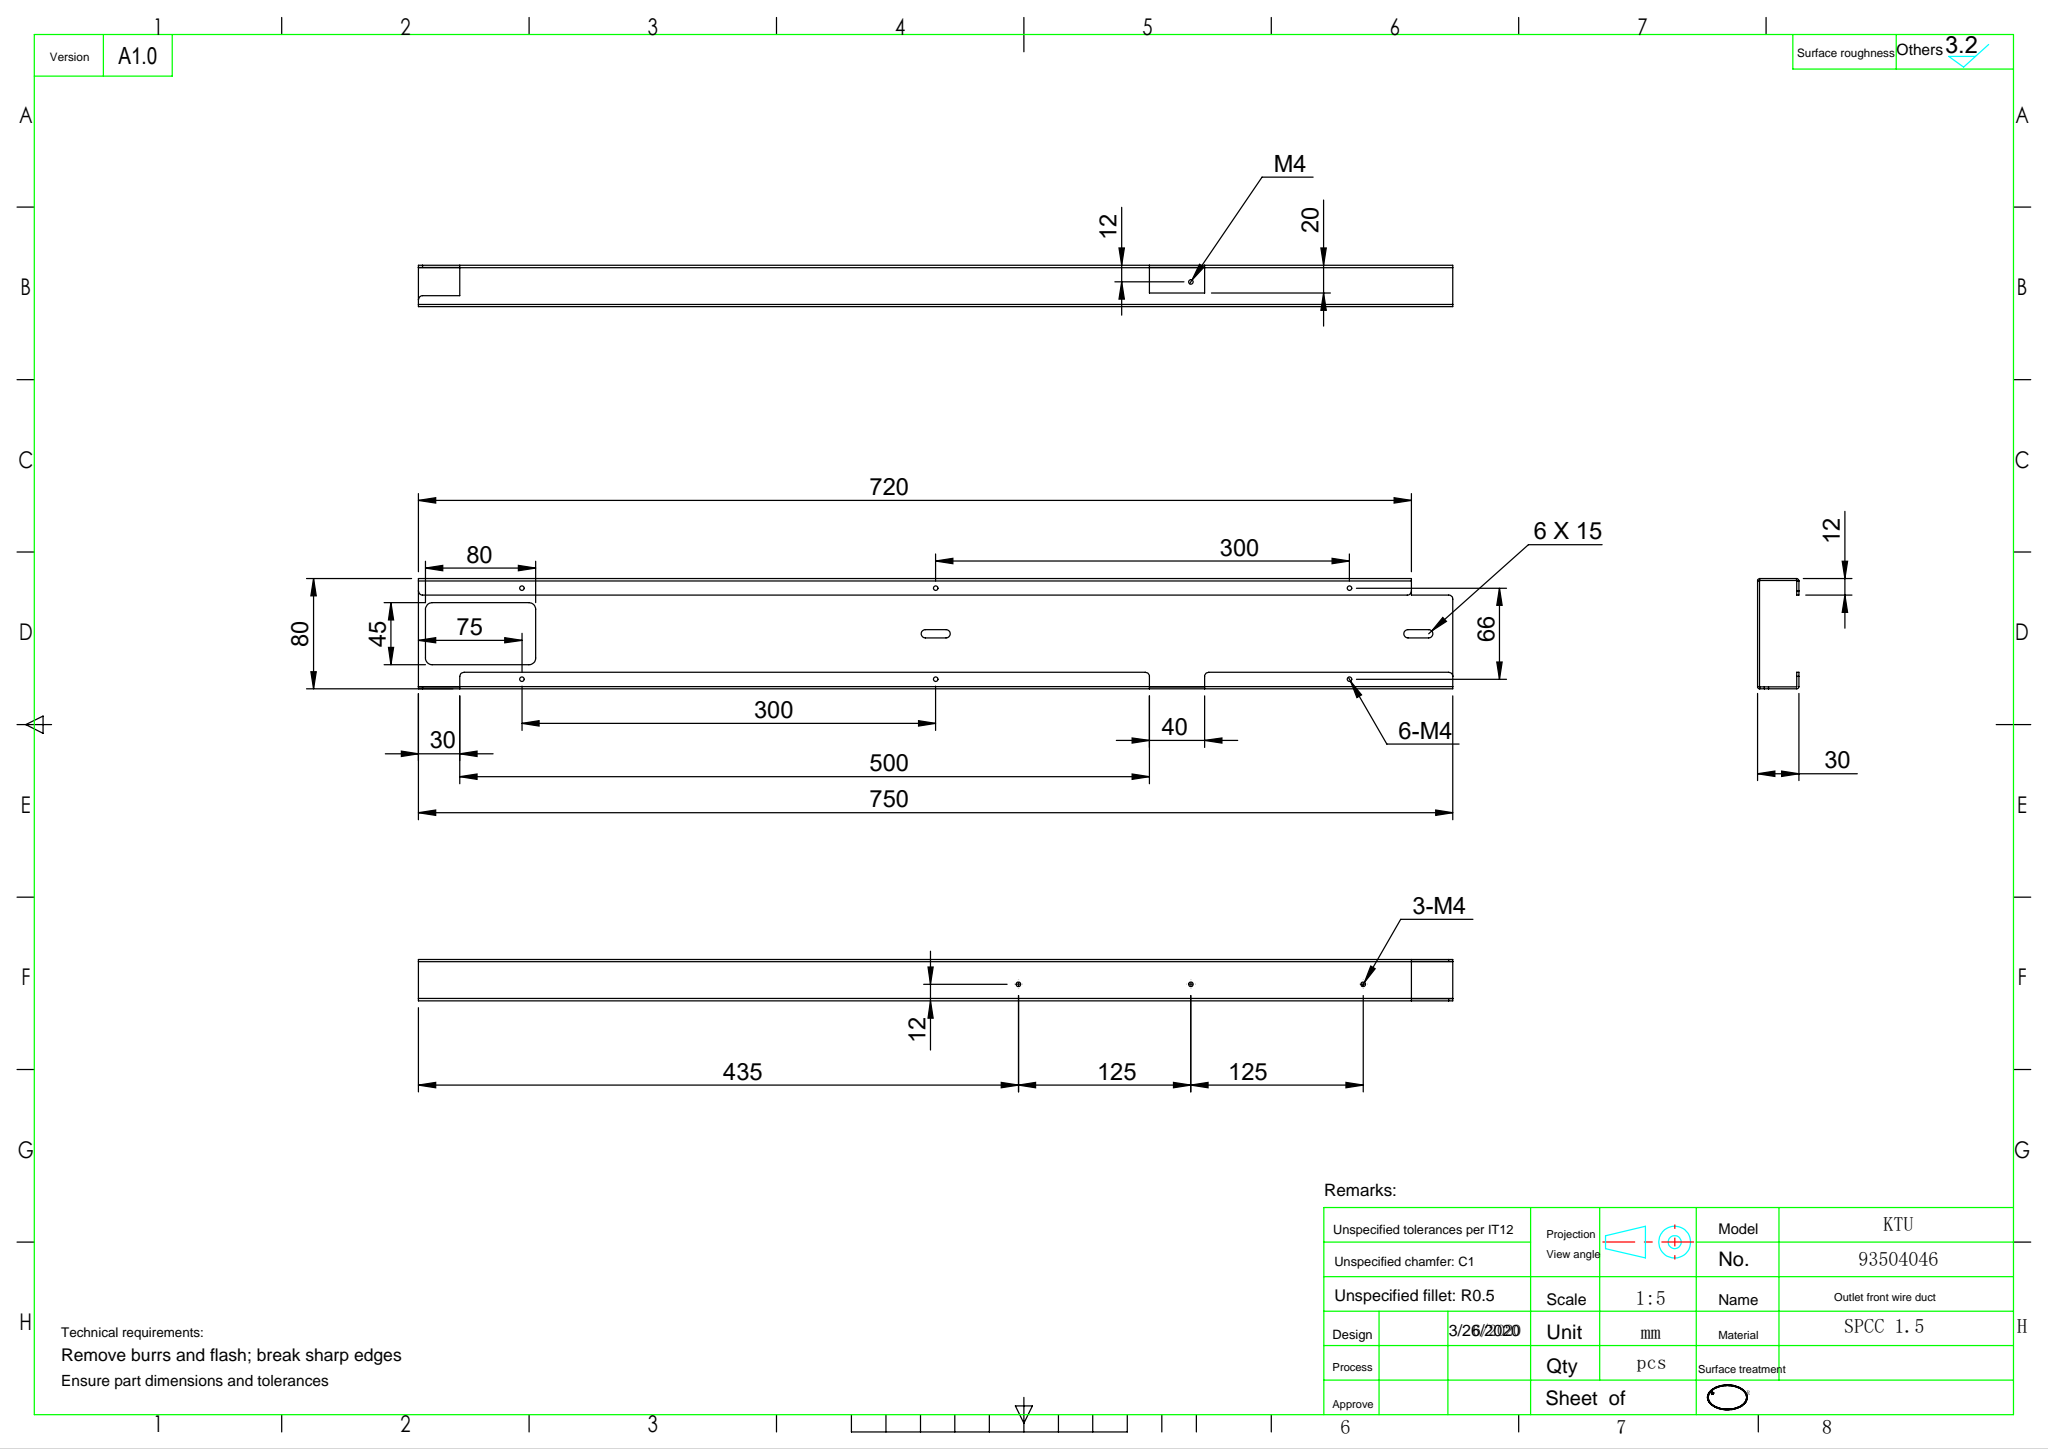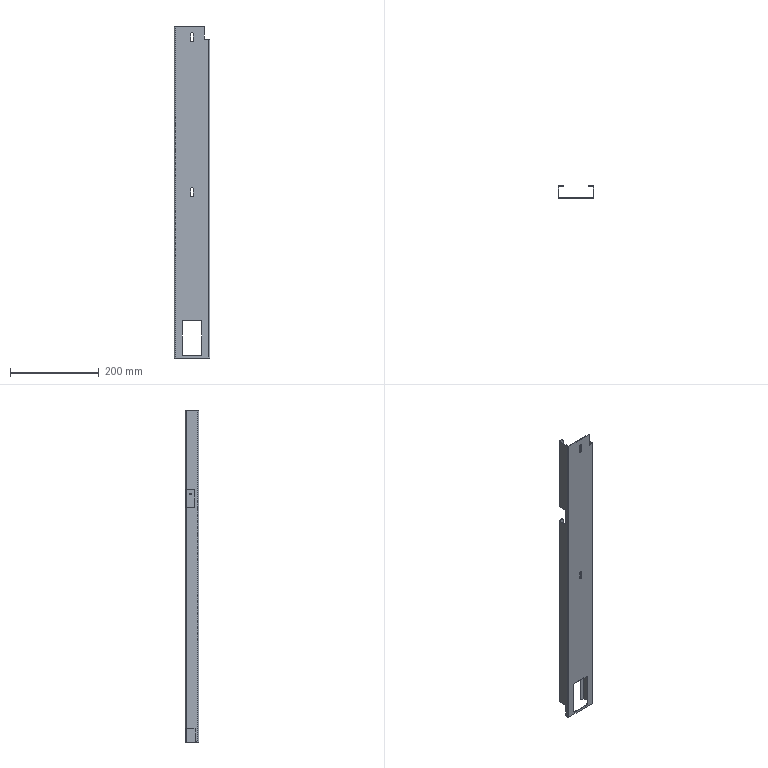Part | SolidWorks | features ICE 5, HoleWzd 2, LPattern 2, Fillet 1, FlatPattern 1, SMBaseFlange 1, SheetMetal 1 | 1 solid | 88 faces | box 80 x 30 x 750 mm | volume 164546 mm3 | cylinder 46 | plane 42 | commonest cylinder face diameters 3.3 x18 6 x14 0.4 x5 3.4 x5 10 x4